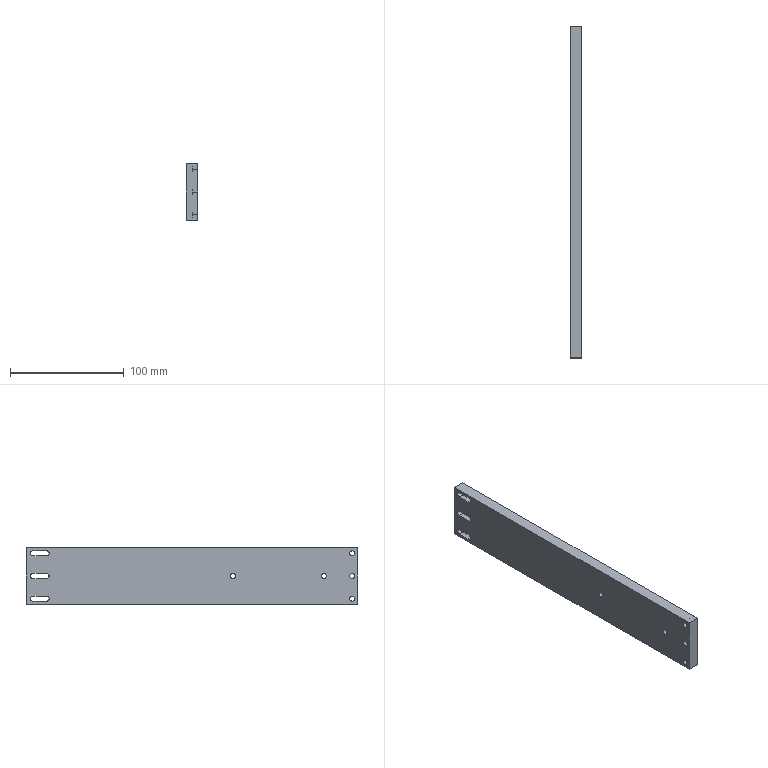Part | STEP file | 04-17 Heat-shrink press cylinder raised bracket plate | 1 solid | 43 faces | box 10 x 292 x 50 mm | volume 141915 mm3 | cylinder 26 | plane 17 | commonest cylinder face diameters 4.5 x16 9 x10